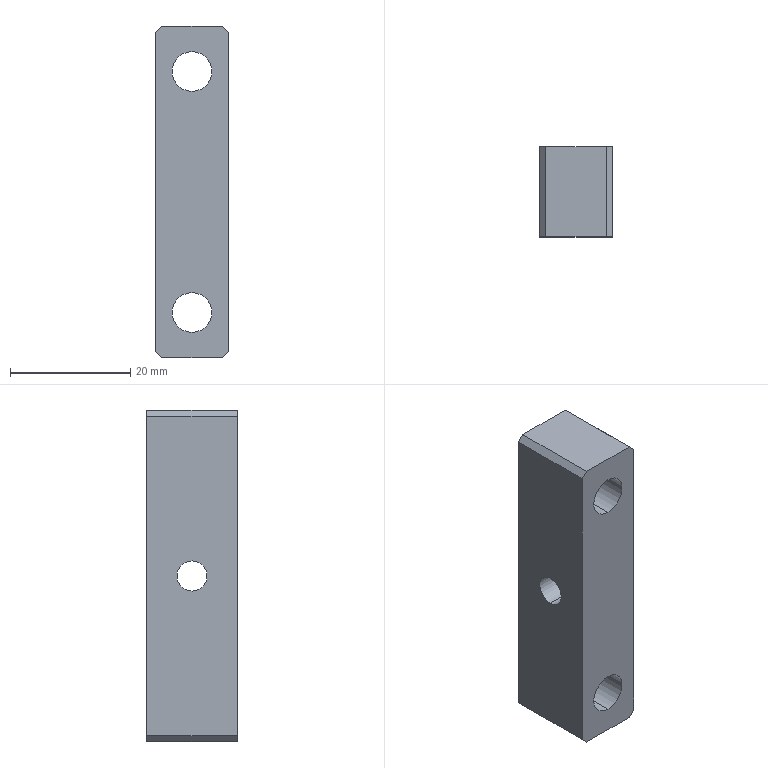Part | SolidWorks | features HoleWzd 2, Chamfer 1, Extrusion 1 | 1 solid | 22 faces | box 12 x 15 x 55 mm | volume 7635 mm3 | plane 12 | cylinder 10 | commonest cylinder face diameters 6.6 x4 11 x4 5 x2
STEP:
#1=CARTESIAN_POINT('',(6.,0.,-2.5));
#2=VERTEX_POINT('',#1);
#3=CARTESIAN_POINT('',(6.,0.,2.5));
#4=VERTEX_POINT('',#3);
#5=CARTESIAN_POINT('',(6.,0.,0.));
#6=DIRECTION('',(-1.,0.,0.));
#7=DIRECTION('',(0.,0.,1.));
#8=AXIS2_PLACEMENT_3D('',#5,#6,#7);
#9=CIRCLE('',#8,2.5);
#10=EDGE_CURVE('',#2,#4,#9,.T.);
#11=ORIENTED_EDGE('',*,*,#10,.F.);
#12=CARTESIAN_POINT('',(-6.,0.,-2.5));
#13=VERTEX_POINT('',#12);
#14=CARTESIAN_POINT('',(-6.,0.,-2.5));
#15=DIRECTION('',(-1.,0.,0.));
#16=VECTOR('',#15,1000.);
#17=LINE('',#14,#16);
#18=EDGE_CURVE('',#2,#13,#17,.T.);
#19=ORIENTED_EDGE('',*,*,#18,.T.);
#20=CARTESIAN_POINT('',(-6.,0.,2.5));
#21=VERTEX_POINT('',#20);
#22=CARTESIAN_POINT('',(-6.,0.,0.));
#23=DIRECTION('',(-1.,0.,0.));
#24=DIRECTION('',(0.,0.,1.));
#25=AXIS2_PLACEMENT_3D('',#22,#23,#24);
#26=CIRCLE('',#25,2.5);
#27=EDGE_CURVE('',#13,#21,#26,.T.);
#28=ORIENTED_EDGE('',*,*,#27,.T.);
#29=CARTESIAN_POINT('',(-6.,0.,2.5));
#30=DIRECTION('',(-1.,0.,0.));
#31=VECTOR('',#30,1000.);
#32=LINE('',#29,#31);
#33=EDGE_CURVE('',#4,#21,#32,.T.);
#34=ORIENTED_EDGE('',*,*,#33,.F.);
#35=EDGE_LOOP('',(#11,#19,#28,#34));
#36=FACE_OUTER_BOUND('',#35,.T.);
#37=CARTESIAN_POINT('',(-6.,0.,0.));
#38=DIRECTION('',(-1.,0.,0.));
#39=DIRECTION('',(0.,0.,1.));
#40=AXIS2_PLACEMENT_3D('',#37,#38,#39);
#41=CYLINDRICAL_SURFACE('',#40,2.5);
#42=ADVANCED_FACE('',(#36),#41,.F.);
#43=CARTESIAN_POINT('',(0.,-0.5,-25.5));
#44=VERTEX_POINT('',#43);
#45=CARTESIAN_POINT('',(0.,-0.5,-14.5));
#46=VERTEX_POINT('',#45);
#47=CARTESIAN_POINT('',(0.,-0.5,-20.));
#48=DIRECTION('',(0.,1.,0.));
#49=DIRECTION('',(0.,0.,1.));
#50=AXIS2_PLACEMENT_3D('',#47,#48,#49);
#51=CIRCLE('',#50,5.5);
#52=EDGE_CURVE('',#44,#46,#51,.T.);
#53=ORIENTED_EDGE('',*,*,#52,.F.);
#54=CARTESIAN_POINT('',(0.,7.5,-25.5));
#55=VERTEX_POINT('',#54);
#56=CARTESIAN_POINT('',(0.,7.5,-25.5));
#57=DIRECTION('',(0.,1.,0.));
#58=VECTOR('',#57,1000.);
#59=LINE('',#56,#58);
#60=EDGE_CURVE('',#44,#55,#59,.T.);
#61=ORIENTED_EDGE('',*,*,#60,.T.);
#62=CARTESIAN_POINT('',(0.,7.5,-14.5));
#63=VERTEX_POINT('',#62);
#64=CARTESIAN_POINT('',(0.,7.5,-20.));
#65=DIRECTION('',(0.,1.,0.));
#66=DIRECTION('',(0.,0.,1.));
#67=AXIS2_PLACEMENT_3D('',#64,#65,#66);
#68=CIRCLE('',#67,5.5);
#69=EDGE_CURVE('',#55,#63,#68,.T.);
#70=ORIENTED_EDGE('',*,*,#69,.T.);
#71=CARTESIAN_POINT('',(0.,7.5,-14.5));
#72=DIRECTION('',(0.,1.,0.));
#73=VECTOR('',#72,1000.);
#74=LINE('',#71,#73);
#75=EDGE_CURVE('',#46,#63,#74,.T.);
#76=ORIENTED_EDGE('',*,*,#75,.F.);
#77=EDGE_LOOP('',(#53,#61,#70,#76));
#78=FACE_OUTER_BOUND('',#77,.T.);
#79=CARTESIAN_POINT('',(0.,7.5,-20.));
#80=DIRECTION('',(0.,1.,0.));
#81=DIRECTION('',(0.,0.,1.));
#82=AXIS2_PLACEMENT_3D('',#79,#80,#81);
#83=CYLINDRICAL_SURFACE('',#82,5.5);
#84=ADVANCED_FACE('',(#78),#83,.F.);
#85=CARTESIAN_POINT('',(0.,-7.5,-16.7));
#86=VERTEX_POINT('',#85);
#87=CARTESIAN_POINT('',(0.,-7.5,-23.3));
#88=VERTEX_POINT('',#87);
#89=CARTESIAN_POINT('',(0.,-7.5,-20.));
#90=DIRECTION('',(0.,-1.,0.));
#91=DIRECTION('',(0.,0.,-1.));
#92=AXIS2_PLACEMENT_3D('',#89,#90,#91);
#93=CIRCLE('',#92,3.3);
#94=EDGE_CURVE('',#86,#88,#93,.T.);
#95=ORIENTED_EDGE('',*,*,#94,.T.);
#96=CARTESIAN_POINT('',(0.,-0.5,-23.3));
#97=VERTEX_POINT('',#96);
#98=CARTESIAN_POINT('',(0.,7.5,-23.3));
#99=DIRECTION('',(0.,1.,0.));
#100=VECTOR('',#99,1000.);
#101=LINE('',#98,#100);
#102=EDGE_CURVE('',#88,#97,#101,.T.);
#103=ORIENTED_EDGE('',*,*,#102,.T.);
#104=CARTESIAN_POINT('',(0.,-0.5,-16.7));
#105=VERTEX_POINT('',#104);
#106=CARTESIAN_POINT('',(0.,-0.5,-20.));
#107=DIRECTION('',(0.,1.,0.));
#108=DIRECTION('',(0.,0.,1.));
#109=AXIS2_PLACEMENT_3D('',#106,#107,#108);
#110=CIRCLE('',#109,3.3);
#111=EDGE_CURVE('',#97,#105,#110,.T.);
#112=ORIENTED_EDGE('',*,*,#111,.T.);
#113=CARTESIAN_POINT('',(0.,7.5,-16.7));
#114=DIRECTION('',(0.,1.,0.));
#115=VECTOR('',#114,1000.);
#116=LINE('',#113,#115);
#117=EDGE_CURVE('',#86,#105,#116,.T.);
#118=ORIENTED_EDGE('',*,*,#117,.F.);
#119=EDGE_LOOP('',(#95,#103,#112,#118));
#120=FACE_OUTER_BOUND('',#119,.T.);
#121=CARTESIAN_POINT('',(0.,7.5,-20.));
#122=DIRECTION('',(0.,1.,0.));
#123=DIRECTION('',(0.,0.,1.));
#124=AXIS2_PLACEMENT_3D('',#121,#122,#123);
#125=CYLINDRICAL_SURFACE('',#124,3.3);
#126=ADVANCED_FACE('',(#120),#125,.F.);
#127=CARTESIAN_POINT('',(0.,-0.5,14.5));
#128=VERTEX_POINT('',#127);
#129=CARTESIAN_POINT('',(0.,-0.5,25.5));
#130=VERTEX_POINT('',#129);
#131=CARTESIAN_POINT('',(0.,-0.5,20.));
#132=DIRECTION('',(0.,1.,0.));
#133=DIRECTION('',(0.,0.,1.));
#134=AXIS2_PLACEMENT_3D('',#131,#132,#133);
#135=CIRCLE('',#134,5.5);
#136=EDGE_CURVE('',#128,#130,#135,.T.);
#137=ORIENTED_EDGE('',*,*,#136,.F.);
#138=CARTESIAN_POINT('',(0.,7.5,14.5));
#139=VERTEX_POINT('',#138);
#140=CARTESIAN_POINT('',(0.,7.5,14.5));
#141=DIRECTION('',(0.,1.,0.));
#142=VECTOR('',#141,1000.);
#143=LINE('',#140,#142);
#144=EDGE_CURVE('',#128,#139,#143,.T.);
#145=ORIENTED_EDGE('',*,*,#144,.T.);
#146=CARTESIAN_POINT('',(0.,7.5,25.5));
#147=VERTEX_POINT('',#146);
#148=CARTESIAN_POINT('',(0.,7.5,20.));
#149=DIRECTION('',(0.,1.,0.));
#150=DIRECTION('',(0.,0.,1.));
#151=AXIS2_PLACEMENT_3D('',#148,#149,#150);
#152=CIRCLE('',#151,5.5);
#153=EDGE_CURVE('',#139,#147,#152,.T.);
#154=ORIENTED_EDGE('',*,*,#153,.T.);
#155=CARTESIAN_POINT('',(0.,7.5,25.5));
#156=DIRECTION('',(0.,1.,0.));
#157=VECTOR('',#156,1000.);
#158=LINE('',#155,#157);
#159=EDGE_CURVE('',#130,#147,#158,.T.);
#160=ORIENTED_EDGE('',*,*,#159,.F.);
#161=EDGE_LOOP('',(#137,#145,#154,#160));
#162=FACE_OUTER_BOUND('',#161,.T.);
#163=CARTESIAN_POINT('',(0.,7.5,20.));
#164=DIRECTION('',(0.,1.,0.));
#165=DIRECTION('',(0.,0.,1.));
#166=AXIS2_PLACEMENT_3D('',#163,#164,#165);
#167=CYLINDRICAL_SURFACE('',#166,5.5);
#168=ADVANCED_FACE('',(#162),#167,.F.);
#169=CARTESIAN_POINT('',(0.,-7.5,23.3));
#170=VERTEX_POINT('',#169);
#171=CARTESIAN_POINT('',(0.,-7.5,16.7));
#172=VERTEX_POINT('',#171);
#173=CARTESIAN_POINT('',(0.,-7.5,20.));
#174=DIRECTION('',(0.,-1.,0.));
#175=DIRECTION('',(0.,0.,-1.));
#176=AXIS2_PLACEMENT_3D('',#173,#174,#175);
#177=CIRCLE('',#176,3.3);
#178=EDGE_CURVE('',#170,#172,#177,.T.);
#179=ORIENTED_EDGE('',*,*,#178,.T.);
#180=CARTESIAN_POINT('',(0.,-0.5,16.7));
#181=VERTEX_POINT('',#180);
#182=CARTESIAN_POINT('',(0.,7.5,16.7));
#183=DIRECTION('',(0.,1.,0.));
#184=VECTOR('',#183,1000.);
#185=LINE('',#182,#184);
#186=EDGE_CURVE('',#172,#181,#185,.T.);
#187=ORIENTED_EDGE('',*,*,#186,.T.);
#188=CARTESIAN_POINT('',(0.,-0.5,23.3));
#189=VERTEX_POINT('',#188);
#190=CARTESIAN_POINT('',(0.,-0.5,20.));
#191=DIRECTION('',(0.,1.,0.));
#192=DIRECTION('',(0.,0.,1.));
#193=AXIS2_PLACEMENT_3D('',#190,#191,#192);
#194=CIRCLE('',#193,3.3);
#195=EDGE_CURVE('',#181,#189,#194,.T.);
#196=ORIENTED_EDGE('',*,*,#195,.T.);
#197=CARTESIAN_POINT('',(0.,7.5,23.3));
#198=DIRECTION('',(0.,1.,0.));
#199=VECTOR('',#198,1000.);
#200=LINE('',#197,#199);
#201=EDGE_CURVE('',#170,#189,#200,.T.);
#202=ORIENTED_EDGE('',*,*,#201,.F.);
#203=EDGE_LOOP('',(#179,#187,#196,#202));
#204=FACE_OUTER_BOUND('',#203,.T.);
#205=CARTESIAN_POINT('',(0.,7.5,20.));
#206=DIRECTION('',(0.,1.,0.));
#207=DIRECTION('',(0.,0.,1.));
#208=AXIS2_PLACEMENT_3D('',#205,#206,#207);
#209=CYLINDRICAL_SURFACE('',#208,3.3);
#210=ADVANCED_FACE('',(#204),#209,.F.);
#211=CARTESIAN_POINT('',(6.,0.,0.));
#212=DIRECTION('',(-1.,0.,0.));
#213=DIRECTION('',(0.,0.,1.));
#214=AXIS2_PLACEMENT_3D('',#211,#212,#213);
#215=CIRCLE('',#214,2.5);
#216=EDGE_CURVE('',#4,#2,#215,.T.);
#217=ORIENTED_EDGE('',*,*,#216,.T.);
#218=ORIENTED_EDGE('',*,*,#10,.T.);
#219=EDGE_LOOP('',(#217,#218));
#220=FACE_BOUND('',#219,.T.);
#221=CARTESIAN_POINT('',(6.,-7.5,26.5));
#222=VERTEX_POINT('',#221);
#223=CARTESIAN_POINT('',(6.,-7.5,-26.5));
#224=VERTEX_POINT('',#223);
#225=CARTESIAN_POINT('',(6.,-7.5,27.5));
#226=DIRECTION('',(0.,0.,-1.));
#227=VECTOR('',#226,1000.);
#228=LINE('',#225,#227);
#229=EDGE_CURVE('',#222,#224,#228,.T.);
#230=ORIENTED_EDGE('',*,*,#229,.T.);
#231=CARTESIAN_POINT('',(6.,7.5,-26.5));
#232=VERTEX_POINT('',#231);
#233=CARTESIAN_POINT('',(6.,7.5,-26.5));
#234=DIRECTION('',(0.,1.,0.));
#235=VECTOR('',#234,1000.);
#236=LINE('',#233,#235);
#237=EDGE_CURVE('',#224,#232,#236,.T.);
#238=ORIENTED_EDGE('',*,*,#237,.T.);
#239=CARTESIAN_POINT('',(6.,7.5,26.5));
#240=VERTEX_POINT('',#239);
#241=CARTESIAN_POINT('',(6.,7.5,27.5));
#242=DIRECTION('',(0.,0.,-1.));
#243=VECTOR('',#242,1000.);
#244=LINE('',#241,#243);
#245=EDGE_CURVE('',#240,#232,#244,.T.);
#246=ORIENTED_EDGE('',*,*,#245,.F.);
#247=CARTESIAN_POINT('',(6.,7.5,26.5));
#248=DIRECTION('',(0.,-1.,0.));
#249=VECTOR('',#248,1000.);
#250=LINE('',#247,#249);
#251=EDGE_CURVE('',#240,#222,#250,.T.);
#252=ORIENTED_EDGE('',*,*,#251,.T.);
#253=EDGE_LOOP('',(#230,#238,#246,#252));
#254=FACE_OUTER_BOUND('',#253,.T.);
#255=CARTESIAN_POINT('',(6.,7.5,27.5));
#256=DIRECTION('',(-1.,0.,0.));
#257=DIRECTION('',(0.,0.,1.));
#258=AXIS2_PLACEMENT_3D('',#255,#256,#257);
#259=PLANE('',#258);
#260=ADVANCED_FACE('',(#220,#254),#259,.F.);
#261=CARTESIAN_POINT('',(5.,7.5,-27.5));
#262=VERTEX_POINT('',#261);
#263=CARTESIAN_POINT('',(-5.,7.5,-27.5));
#264=VERTEX_POINT('',#263);
#265=CARTESIAN_POINT('',(-6.,7.5,-27.5));
#266=DIRECTION('',(-1.,0.,0.));
#267=VECTOR('',#266,1000.);
#268=LINE('',#265,#267);
#269=EDGE_CURVE('',#262,#264,#268,.T.);
#270=ORIENTED_EDGE('',*,*,#269,.F.);
#271=CARTESIAN_POINT('',(5.,-7.5,-27.5));
#272=VERTEX_POINT('',#271);
#273=CARTESIAN_POINT('',(5.,7.5,-27.5));
#274=DIRECTION('',(0.,-1.,0.));
#275=VECTOR('',#274,1000.);
#276=LINE('',#273,#275);
#277=EDGE_CURVE('',#262,#272,#276,.T.);
#278=ORIENTED_EDGE('',*,*,#277,.T.);
#279=CARTESIAN_POINT('',(-5.,-7.5,-27.5));
#280=VERTEX_POINT('',#279);
#281=CARTESIAN_POINT('',(-6.,-7.5,-27.5));
#282=DIRECTION('',(-1.,0.,0.));
#283=VECTOR('',#282,1000.);
#284=LINE('',#281,#283);
#285=EDGE_CURVE('',#272,#280,#284,.T.);
#286=ORIENTED_EDGE('',*,*,#285,.T.);
#287=CARTESIAN_POINT('',(-5.,7.5,-27.5));
#288=DIRECTION('',(0.,1.,0.));
#289=VECTOR('',#288,1000.);
#290=LINE('',#287,#289);
#291=EDGE_CURVE('',#280,#264,#290,.T.);
#292=ORIENTED_EDGE('',*,*,#291,.T.);
#293=EDGE_LOOP('',(#270,#278,#286,#292));
#294=FACE_OUTER_BOUND('',#293,.T.);
#295=CARTESIAN_POINT('',(-6.,7.5,-27.5));
#296=DIRECTION('',(0.,0.,1.));
#297=DIRECTION('',(1.,0.,0.));
#298=AXIS2_PLACEMENT_3D('',#295,#296,#297);
#299=PLANE('',#298);
#300=ADVANCED_FACE('',(#294),#299,.F.);
#301=CARTESIAN_POINT('',(-6.,0.,0.));
#302=DIRECTION('',(-1.,0.,0.));
#303=DIRECTION('',(0.,0.,1.));
#304=AXIS2_PLACEMENT_3D('',#301,#302,#303);
#305=CIRCLE('',#304,2.5);
#306=EDGE_CURVE('',#21,#13,#305,.T.);
#307=ORIENTED_EDGE('',*,*,#306,.F.);
#308=ORIENTED_EDGE('',*,*,#27,.F.);
#309=EDGE_LOOP('',(#307,#308));
#310=FACE_BOUND('',#309,.T.);
#311=CARTESIAN_POINT('',(-6.,7.5,-26.5));
#312=VERTEX_POINT('',#311);
#313=CARTESIAN_POINT('',(-6.,7.5,26.5));
#314=VERTEX_POINT('',#313);
#315=CARTESIAN_POINT('',(-6.,7.5,27.5));
#316=DIRECTION('',(0.,0.,1.));
#317=VECTOR('',#316,1000.);
#318=LINE('',#315,#317);
#319=EDGE_CURVE('',#312,#314,#318,.T.);
#320=ORIENTED_EDGE('',*,*,#319,.F.);
#321=CARTESIAN_POINT('',(-6.,-7.5,-26.5));
#322=VERTEX_POINT('',#321);
#323=CARTESIAN_POINT('',(-6.,7.5,-26.5));
#324=DIRECTION('',(0.,-1.,0.));
#325=VECTOR('',#324,1000.);
#326=LINE('',#323,#325);
#327=EDGE_CURVE('',#312,#322,#326,.T.);
#328=ORIENTED_EDGE('',*,*,#327,.T.);
#329=CARTESIAN_POINT('',(-6.,-7.5,26.5));
#330=VERTEX_POINT('',#329);
#331=CARTESIAN_POINT('',(-6.,-7.5,27.5));
#332=DIRECTION('',(0.,0.,1.));
#333=VECTOR('',#332,1000.);
#334=LINE('',#331,#333);
#335=EDGE_CURVE('',#322,#330,#334,.T.);
#336=ORIENTED_EDGE('',*,*,#335,.T.);
#337=CARTESIAN_POINT('',(-6.,7.5,26.5));
#338=DIRECTION('',(0.,1.,0.));
#339=VECTOR('',#338,1000.);
#340=LINE('',#337,#339);
#341=EDGE_CURVE('',#330,#314,#340,.T.);
#342=ORIENTED_EDGE('',*,*,#341,.T.);
#343=EDGE_LOOP('',(#320,#328,#336,#342));
#344=FACE_OUTER_BOUND('',#343,.T.);
#345=CARTESIAN_POINT('',(-6.,7.5,27.5));
#346=DIRECTION('',(1.,0.,0.));
#347=DIRECTION('',(0.,0.,-1.));
#348=AXIS2_PLACEMENT_3D('',#345,#346,#347);
#349=PLANE('',#348);
#350=ADVANCED_FACE('',(#310,#344),#349,.F.);
#351=CARTESIAN_POINT('',(-5.,-7.5,27.5));
#352=VERTEX_POINT('',#351);
#353=CARTESIAN_POINT('',(5.,-7.5,27.5));
#354=VERTEX_POINT('',#353);
#355=CARTESIAN_POINT('',(-6.,-7.5,27.5));
#356=DIRECTION('',(1.,0.,0.));
#357=VECTOR('',#356,1000.);
#358=LINE('',#355,#357);
#359=EDGE_CURVE('',#352,#354,#358,.T.);
#360=ORIENTED_EDGE('',*,*,#359,.T.);
#361=CARTESIAN_POINT('',(5.,7.5,27.5));
#362=VERTEX_POINT('',#361);
#363=CARTESIAN_POINT('',(5.,7.5,27.5));
#364=DIRECTION('',(0.,1.,0.));
#365=VECTOR('',#364,1000.);
#366=LINE('',#363,#365);
#367=EDGE_CURVE('',#354,#362,#366,.T.);
#368=ORIENTED_EDGE('',*,*,#367,.T.);
#369=CARTESIAN_POINT('',(-5.,7.5,27.5));
#370=VERTEX_POINT('',#369);
#371=CARTESIAN_POINT('',(-6.,7.5,27.5));
#372=DIRECTION('',(1.,0.,0.));
#373=VECTOR('',#372,1000.);
#374=LINE('',#371,#373);
#375=EDGE_CURVE('',#370,#362,#374,.T.);
#376=ORIENTED_EDGE('',*,*,#375,.F.);
#377=CARTESIAN_POINT('',(-5.,7.5,27.5));
#378=DIRECTION('',(0.,-1.,0.));
#379=VECTOR('',#378,1000.);
#380=LINE('',#377,#379);
#381=EDGE_CURVE('',#370,#352,#380,.T.);
#382=ORIENTED_EDGE('',*,*,#381,.T.);
#383=EDGE_LOOP('',(#360,#368,#376,#382));
#384=FACE_OUTER_BOUND('',#383,.T.);
#385=CARTESIAN_POINT('',(-6.,7.5,27.5));
#386=DIRECTION('',(0.,0.,-1.));
#387=DIRECTION('',(-1.,0.,0.));
#388=AXIS2_PLACEMENT_3D('',#385,#386,#387);
#389=PLANE('',#388);
#390=ADVANCED_FACE('',(#384),#389,.F.);
#391=CARTESIAN_POINT('',(0.,7.5,-20.));
#392=DIRECTION('',(0.,1.,0.));
#393=DIRECTION('',(0.,0.,1.));
#394=AXIS2_PLACEMENT_3D('',#391,#392,#393);
#395=CIRCLE('',#394,5.5);
#396=EDGE_CURVE('',#63,#55,#395,.T.);
#397=ORIENTED_EDGE('',*,*,#396,.F.);
#398=ORIENTED_EDGE('',*,*,#69,.F.);
#399=EDGE_LOOP('',(#397,#398));
#400=FACE_BOUND('',#399,.T.);
#401=CARTESIAN_POINT('',(0.,7.5,20.));
#402=DIRECTION('',(0.,1.,0.));
#403=DIRECTION('',(0.,0.,1.));
#404=AXIS2_PLACEMENT_3D('',#401,#402,#403);
#405=CIRCLE('',#404,5.5);
#406=EDGE_CURVE('',#147,#139,#405,.T.);
#407=ORIENTED_EDGE('',*,*,#406,.F.);
#408=ORIENTED_EDGE('',*,*,#153,.F.);
#409=EDGE_LOOP('',(#407,#408));
#410=FACE_BOUND('',#409,.T.);
#411=ORIENTED_EDGE('',*,*,#245,.T.);
#412=CARTESIAN_POINT('',(5.,7.5,-27.5));
#413=DIRECTION('',(-0.7071,0.,-0.7071));
#414=VECTOR('',#413,1000.);
#415=LINE('',#412,#414);
#416=EDGE_CURVE('',#232,#262,#415,.T.);
#417=ORIENTED_EDGE('',*,*,#416,.T.);
#418=ORIENTED_EDGE('',*,*,#269,.T.);
#419=CARTESIAN_POINT('',(-6.,7.5,-26.5));
#420=DIRECTION('',(-0.7071,0.,0.7071));
#421=VECTOR('',#420,1000.);
#422=LINE('',#419,#421);
#423=EDGE_CURVE('',#264,#312,#422,.T.);
#424=ORIENTED_EDGE('',*,*,#423,.T.);
#425=ORIENTED_EDGE('',*,*,#319,.T.);
#426=CARTESIAN_POINT('',(-5.,7.5,27.5));
#427=DIRECTION('',(0.7071,0.,0.7071));
#428=VECTOR('',#427,1000.);
#429=LINE('',#426,#428);
#430=EDGE_CURVE('',#314,#370,#429,.T.);
#431=ORIENTED_EDGE('',*,*,#430,.T.);
#432=ORIENTED_EDGE('',*,*,#375,.T.);
#433=CARTESIAN_POINT('',(6.,7.5,26.5));
#434=DIRECTION('',(0.7071,0.,-0.7071));
#435=VECTOR('',#434,1000.);
#436=LINE('',#433,#435);
#437=EDGE_CURVE('',#362,#240,#436,.T.);
#438=ORIENTED_EDGE('',*,*,#437,.T.);
#439=EDGE_LOOP('',(#411,#417,#418,#424,#425,#431,#432,#438));
#440=FACE_OUTER_BOUND('',#439,.T.);
#441=CARTESIAN_POINT('',(0.,7.5,0.));
#442=DIRECTION('',(0.,-1.,0.));
#443=DIRECTION('',(0.,0.,-1.));
#444=AXIS2_PLACEMENT_3D('',#441,#442,#443);
#445=PLANE('',#444);
#446=ADVANCED_FACE('',(#400,#410,#440),#445,.F.);
#447=ORIENTED_EDGE('',*,*,#94,.F.);
#448=CARTESIAN_POINT('',(0.,-7.5,-20.));
#449=DIRECTION('',(0.,-1.,0.));
#450=DIRECTION('',(0.,0.,-1.));
#451=AXIS2_PLACEMENT_3D('',#448,#449,#450);
#452=CIRCLE('',#451,3.3);
#453=EDGE_CURVE('',#88,#86,#452,.T.);
#454=ORIENTED_EDGE('',*,*,#453,.F.);
#455=EDGE_LOOP('',(#447,#454));
#456=FACE_BOUND('',#455,.T.);
#457=ORIENTED_EDGE('',*,*,#178,.F.);
#458=CARTESIAN_POINT('',(0.,-7.5,20.));
#459=DIRECTION('',(0.,-1.,0.));
#460=DIRECTION('',(0.,0.,-1.));
#461=AXIS2_PLACEMENT_3D('',#458,#459,#460);
#462=CIRCLE('',#461,3.3);
#463=EDGE_CURVE('',#172,#170,#462,.T.);
#464=ORIENTED_EDGE('',*,*,#463,.F.);
#465=EDGE_LOOP('',(#457,#464));
#466=FACE_BOUND('',#465,.T.);
#467=ORIENTED_EDGE('',*,*,#285,.F.);
#468=CARTESIAN_POINT('',(16.25,-7.5,-16.25));
#469=DIRECTION('',(0.7071,0.,0.7071));
#470=VECTOR('',#469,1000.);
#471=LINE('',#468,#470);
#472=EDGE_CURVE('',#272,#224,#471,.T.);
#473=ORIENTED_EDGE('',*,*,#472,.T.);
#474=ORIENTED_EDGE('',*,*,#229,.F.);
#475=CARTESIAN_POINT('',(16.25,-7.5,16.25));
#476=DIRECTION('',(-0.7071,0.,0.7071));
#477=VECTOR('',#476,1000.);
#478=LINE('',#475,#477);
#479=EDGE_CURVE('',#222,#354,#478,.T.);
#480=ORIENTED_EDGE('',*,*,#479,.T.);
#481=ORIENTED_EDGE('',*,*,#359,.F.);
#482=CARTESIAN_POINT('',(-16.25,-7.5,16.25));
#483=DIRECTION('',(-0.7071,0.,-0.7071));
#484=VECTOR('',#483,1000.);
#485=LINE('',#482,#484);
#486=EDGE_CURVE('',#352,#330,#485,.T.);
#487=ORIENTED_EDGE('',*,*,#486,.T.);
#488=ORIENTED_EDGE('',*,*,#335,.F.);
#489=CARTESIAN_POINT('',(-16.25,-7.5,-16.25));
#490=DIRECTION('',(0.7071,0.,-0.7071));
#491=VECTOR('',#490,1000.);
#492=LINE('',#489,#491);
#493=EDGE_CURVE('',#322,#280,#492,.T.);
#494=ORIENTED_EDGE('',*,*,#493,.T.);
#495=EDGE_LOOP('',(#467,#473,#474,#480,#481,#487,#488,#494));
#496=FACE_OUTER_BOUND('',#495,.T.);
#497=CARTESIAN_POINT('',(0.,-7.5,0.));
#498=DIRECTION('',(0.,-1.,0.));
#499=DIRECTION('',(0.,0.,-1.));
#500=AXIS2_PLACEMENT_3D('',#497,#498,#499);
#501=PLANE('',#500);
#502=ADVANCED_FACE('',(#456,#466,#496),#501,.T.);
#503=ORIENTED_EDGE('',*,*,#416,.F.);
#504=ORIENTED_EDGE('',*,*,#237,.F.);
#505=ORIENTED_EDGE('',*,*,#472,.F.);
#506=ORIENTED_EDGE('',*,*,#277,.F.);
#507=EDGE_LOOP('',(#503,#504,#505,#506));
#508=FACE_OUTER_BOUND('',#507,.T.);
#509=CARTESIAN_POINT('',(5.,7.5,-27.5));
#510=DIRECTION('',(-0.7071,0.,0.7071));
#511=DIRECTION('',(0.,-1.,0.));
#512=AXIS2_PLACEMENT_3D('',#509,#510,#511);
#513=PLANE('',#512);
#514=ADVANCED_FACE('',(#508),#513,.F.);
#515=ORIENTED_EDGE('',*,*,#423,.F.);
#516=ORIENTED_EDGE('',*,*,#291,.F.);
#517=ORIENTED_EDGE('',*,*,#493,.F.);
#518=ORIENTED_EDGE('',*,*,#327,.F.);
#519=EDGE_LOOP('',(#515,#516,#517,#518));
#520=FACE_OUTER_BOUND('',#519,.T.);
#521=CARTESIAN_POINT('',(-6.,7.5,-26.5));
#522=DIRECTION('',(0.7071,0.,0.7071));
#523=DIRECTION('',(0.,-1.,0.));
#524=AXIS2_PLACEMENT_3D('',#521,#522,#523);
#525=PLANE('',#524);
#526=ADVANCED_FACE('',(#520),#525,.F.);
#527=ORIENTED_EDGE('',*,*,#437,.F.);
#528=ORIENTED_EDGE('',*,*,#367,.F.);
#529=ORIENTED_EDGE('',*,*,#479,.F.);
#530=ORIENTED_EDGE('',*,*,#251,.F.);
#531=EDGE_LOOP('',(#527,#528,#529,#530));
#532=FACE_OUTER_BOUND('',#531,.T.);
#533=CARTESIAN_POINT('',(6.,7.5,26.5));
#534=DIRECTION('',(-0.7071,0.,-0.7071));
#535=DIRECTION('',(0.,-1.,0.));
#536=AXIS2_PLACEMENT_3D('',#533,#534,#535);
#537=PLANE('',#536);
#538=ADVANCED_FACE('',(#532),#537,.F.);
#539=ORIENTED_EDGE('',*,*,#430,.F.);
#540=ORIENTED_EDGE('',*,*,#341,.F.);
#541=ORIENTED_EDGE('',*,*,#486,.F.);
#542=ORIENTED_EDGE('',*,*,#381,.F.);
#543=EDGE_LOOP('',(#539,#540,#541,#542));
#544=FACE_OUTER_BOUND('',#543,.T.);
#545=CARTESIAN_POINT('',(-5.,7.5,27.5));
#546=DIRECTION('',(0.7071,0.,-0.7071));
#547=DIRECTION('',(0.,-1.,0.));
#548=AXIS2_PLACEMENT_3D('',#545,#546,#547);
#549=PLANE('',#548);
#550=ADVANCED_FACE('',(#544),#549,.F.);
#551=ORIENTED_EDGE('',*,*,#186,.F.);
#552=ORIENTED_EDGE('',*,*,#463,.T.);
#553=ORIENTED_EDGE('',*,*,#201,.T.);
#554=CARTESIAN_POINT('',(0.,-0.5,20.));
#555=DIRECTION('',(0.,1.,0.));
#556=DIRECTION('',(0.,0.,1.));
#557=AXIS2_PLACEMENT_3D('',#554,#555,#556);
#558=CIRCLE('',#557,3.3);
#559=EDGE_CURVE('',#189,#181,#558,.T.);
#560=ORIENTED_EDGE('',*,*,#559,.T.);
#561=EDGE_LOOP('',(#551,#552,#553,#560));
#562=FACE_OUTER_BOUND('',#561,.T.);
#563=CARTESIAN_POINT('',(0.,7.5,20.));
#564=DIRECTION('',(0.,1.,0.));
#565=DIRECTION('',(0.,0.,1.));
#566=AXIS2_PLACEMENT_3D('',#563,#564,#565);
#567=CYLINDRICAL_SURFACE('',#566,3.3);
#568=ADVANCED_FACE('',(#562),#567,.F.);
#569=ORIENTED_EDGE('',*,*,#559,.F.);
#570=ORIENTED_EDGE('',*,*,#195,.F.);
#571=EDGE_LOOP('',(#569,#570));
#572=FACE_BOUND('',#571,.T.);
#573=CARTESIAN_POINT('',(0.,-0.5,20.));
#574=DIRECTION('',(0.,1.,0.));
#575=DIRECTION('',(0.,0.,1.));
#576=AXIS2_PLACEMENT_3D('',#573,#574,#575);
#577=CIRCLE('',#576,5.5);
#578=EDGE_CURVE('',#130,#128,#577,.T.);
#579=ORIENTED_EDGE('',*,*,#578,.T.);
#580=ORIENTED_EDGE('',*,*,#136,.T.);
#581=EDGE_LOOP('',(#579,#580));
#582=FACE_OUTER_BOUND('',#581,.T.);
#583=CARTESIAN_POINT('',(3.3,-0.5,20.));
#584=DIRECTION('',(0.,-1.,0.));
#585=DIRECTION('',(0.,0.,-1.));
#586=AXIS2_PLACEMENT_3D('',#583,#584,#585);
#587=PLANE('',#586);
#588=ADVANCED_FACE('',(#572,#582),#587,.F.);
#589=ORIENTED_EDGE('',*,*,#144,.F.);
#590=ORIENTED_EDGE('',*,*,#578,.F.);
#591=ORIENTED_EDGE('',*,*,#159,.T.);
#592=ORIENTED_EDGE('',*,*,#406,.T.);
#593=EDGE_LOOP('',(#589,#590,#591,#592));
#594=FACE_OUTER_BOUND('',#593,.T.);
#595=CARTESIAN_POINT('',(0.,7.5,20.));
#596=DIRECTION('',(0.,1.,0.));
#597=DIRECTION('',(0.,0.,1.));
#598=AXIS2_PLACEMENT_3D('',#595,#596,#597);
#599=CYLINDRICAL_SURFACE('',#598,5.5);
#600=ADVANCED_FACE('',(#594),#599,.F.);
#601=ORIENTED_EDGE('',*,*,#102,.F.);
#602=ORIENTED_EDGE('',*,*,#453,.T.);
#603=ORIENTED_EDGE('',*,*,#117,.T.);
#604=CARTESIAN_POINT('',(0.,-0.5,-20.));
#605=DIRECTION('',(0.,1.,0.));
#606=DIRECTION('',(0.,0.,1.));
#607=AXIS2_PLACEMENT_3D('',#604,#605,#606);
#608=CIRCLE('',#607,3.3);
#609=EDGE_CURVE('',#105,#97,#608,.T.);
#610=ORIENTED_EDGE('',*,*,#609,.T.);
#611=EDGE_LOOP('',(#601,#602,#603,#610));
#612=FACE_OUTER_BOUND('',#611,.T.);
#613=CARTESIAN_POINT('',(0.,7.5,-20.));
#614=DIRECTION('',(0.,1.,0.));
#615=DIRECTION('',(0.,0.,1.));
#616=AXIS2_PLACEMENT_3D('',#613,#614,#615);
#617=CYLINDRICAL_SURFACE('',#616,3.3);
#618=ADVANCED_FACE('',(#612),#617,.F.);
#619=ORIENTED_EDGE('',*,*,#609,.F.);
#620=ORIENTED_EDGE('',*,*,#111,.F.);
#621=EDGE_LOOP('',(#619,#620));
#622=FACE_BOUND('',#621,.T.);
#623=CARTESIAN_POINT('',(0.,-0.5,-20.));
#624=DIRECTION('',(0.,1.,0.));
#625=DIRECTION('',(0.,0.,1.));
#626=AXIS2_PLACEMENT_3D('',#623,#624,#625);
#627=CIRCLE('',#626,5.5);
#628=EDGE_CURVE('',#46,#44,#627,.T.);
#629=ORIENTED_EDGE('',*,*,#628,.T.);
#630=ORIENTED_EDGE('',*,*,#52,.T.);
#631=EDGE_LOOP('',(#629,#630));
#632=FACE_OUTER_BOUND('',#631,.T.);
#633=CARTESIAN_POINT('',(3.3,-0.5,-20.));
#634=DIRECTION('',(0.,-1.,0.));
#635=DIRECTION('',(0.,0.,-1.));
#636=AXIS2_PLACEMENT_3D('',#633,#634,#635);
#637=PLANE('',#636);
#638=ADVANCED_FACE('',(#622,#632),#637,.F.);
#639=ORIENTED_EDGE('',*,*,#60,.F.);
#640=ORIENTED_EDGE('',*,*,#628,.F.);
#641=ORIENTED_EDGE('',*,*,#75,.T.);
#642=ORIENTED_EDGE('',*,*,#396,.T.);
#643=EDGE_LOOP('',(#639,#640,#641,#642));
#644=FACE_OUTER_BOUND('',#643,.T.);
#645=CARTESIAN_POINT('',(0.,7.5,-20.));
#646=DIRECTION('',(0.,1.,0.));
#647=DIRECTION('',(0.,0.,1.));
#648=AXIS2_PLACEMENT_3D('',#645,#646,#647);
#649=CYLINDRICAL_SURFACE('',#648,5.5);
#650=ADVANCED_FACE('',(#644),#649,.F.);
#651=ORIENTED_EDGE('',*,*,#18,.F.);
#652=ORIENTED_EDGE('',*,*,#216,.F.);
#653=ORIENTED_EDGE('',*,*,#33,.T.);
#654=ORIENTED_EDGE('',*,*,#306,.T.);
#655=EDGE_LOOP('',(#651,#652,#653,#654));
#656=FACE_OUTER_BOUND('',#655,.T.);
#657=CARTESIAN_POINT('',(-6.,0.,0.));
#658=DIRECTION('',(-1.,0.,0.));
#659=DIRECTION('',(0.,0.,1.));
#660=AXIS2_PLACEMENT_3D('',#657,#658,#659);
#661=CYLINDRICAL_SURFACE('',#660,2.5);
#662=ADVANCED_FACE('',(#656),#661,.F.);
#663=CLOSED_SHELL('',(#42,#84,#126,#168,#210,#260,#300,#350,#390,#446,#502,#514,#526,#538,#550,#568,#588,#600,#618,#638,#650,#662));
#664=MANIFOLD_SOLID_BREP('',#663);
#665=CARTESIAN_POINT('',(0.,0.,0.));
#666=DIRECTION('',(0.,0.,1.));
#667=DIRECTION('',(1.,0.,0.));
#668=AXIS2_PLACEMENT_3D('',#665,#666,#667);
#669=(LENGTH_UNIT()NAMED_UNIT(*)SI_UNIT(.MILLI.,.METRE.));
#670=UNCERTAINTY_MEASURE_WITH_UNIT(LENGTH_MEASURE(0.00001),#669,'','');
#671=(NAMED_UNIT(*)PLANE_ANGLE_UNIT()SI_UNIT($,.RADIAN.));
#672=(NAMED_UNIT(*)SI_UNIT($,.STERADIAN.)SOLID_ANGLE_UNIT());
#673=(GEOMETRIC_REPRESENTATION_CONTEXT(3)GLOBAL_UNCERTAINTY_ASSIGNED_CONTEXT((#670))GLOBAL_UNIT_ASSIGNED_CONTEXT((#669,#671,#672))REPRESENTATION_CONTEXT('',''));
#674=ADVANCED_BREP_SHAPE_REPRESENTATION('',(#664,#668),#673);